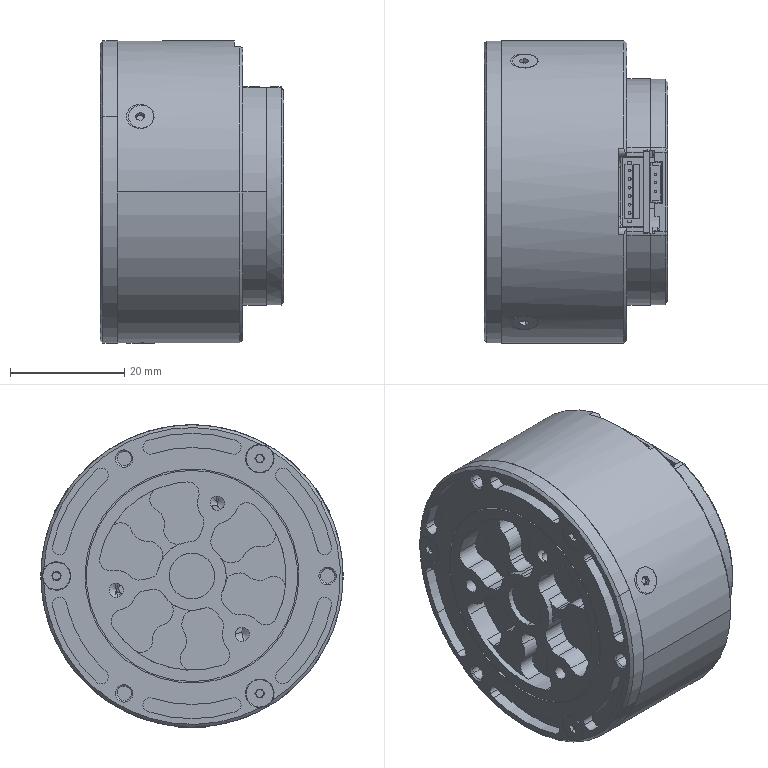Part | SolidWorks | features ICE 1, MBimport 1 | 31 solids | 1263 faces | box 32.2 x 53 x 53 mm | volume 55104 mm3 | plane 563 | cylinder 453 | cone 131 | spline 102 | torus 10 | sphere 4 | commonest cylinder face diameters 4 x66 2.5 x54 0.5 x48 2 x22 4.5 x18 0.1 x16